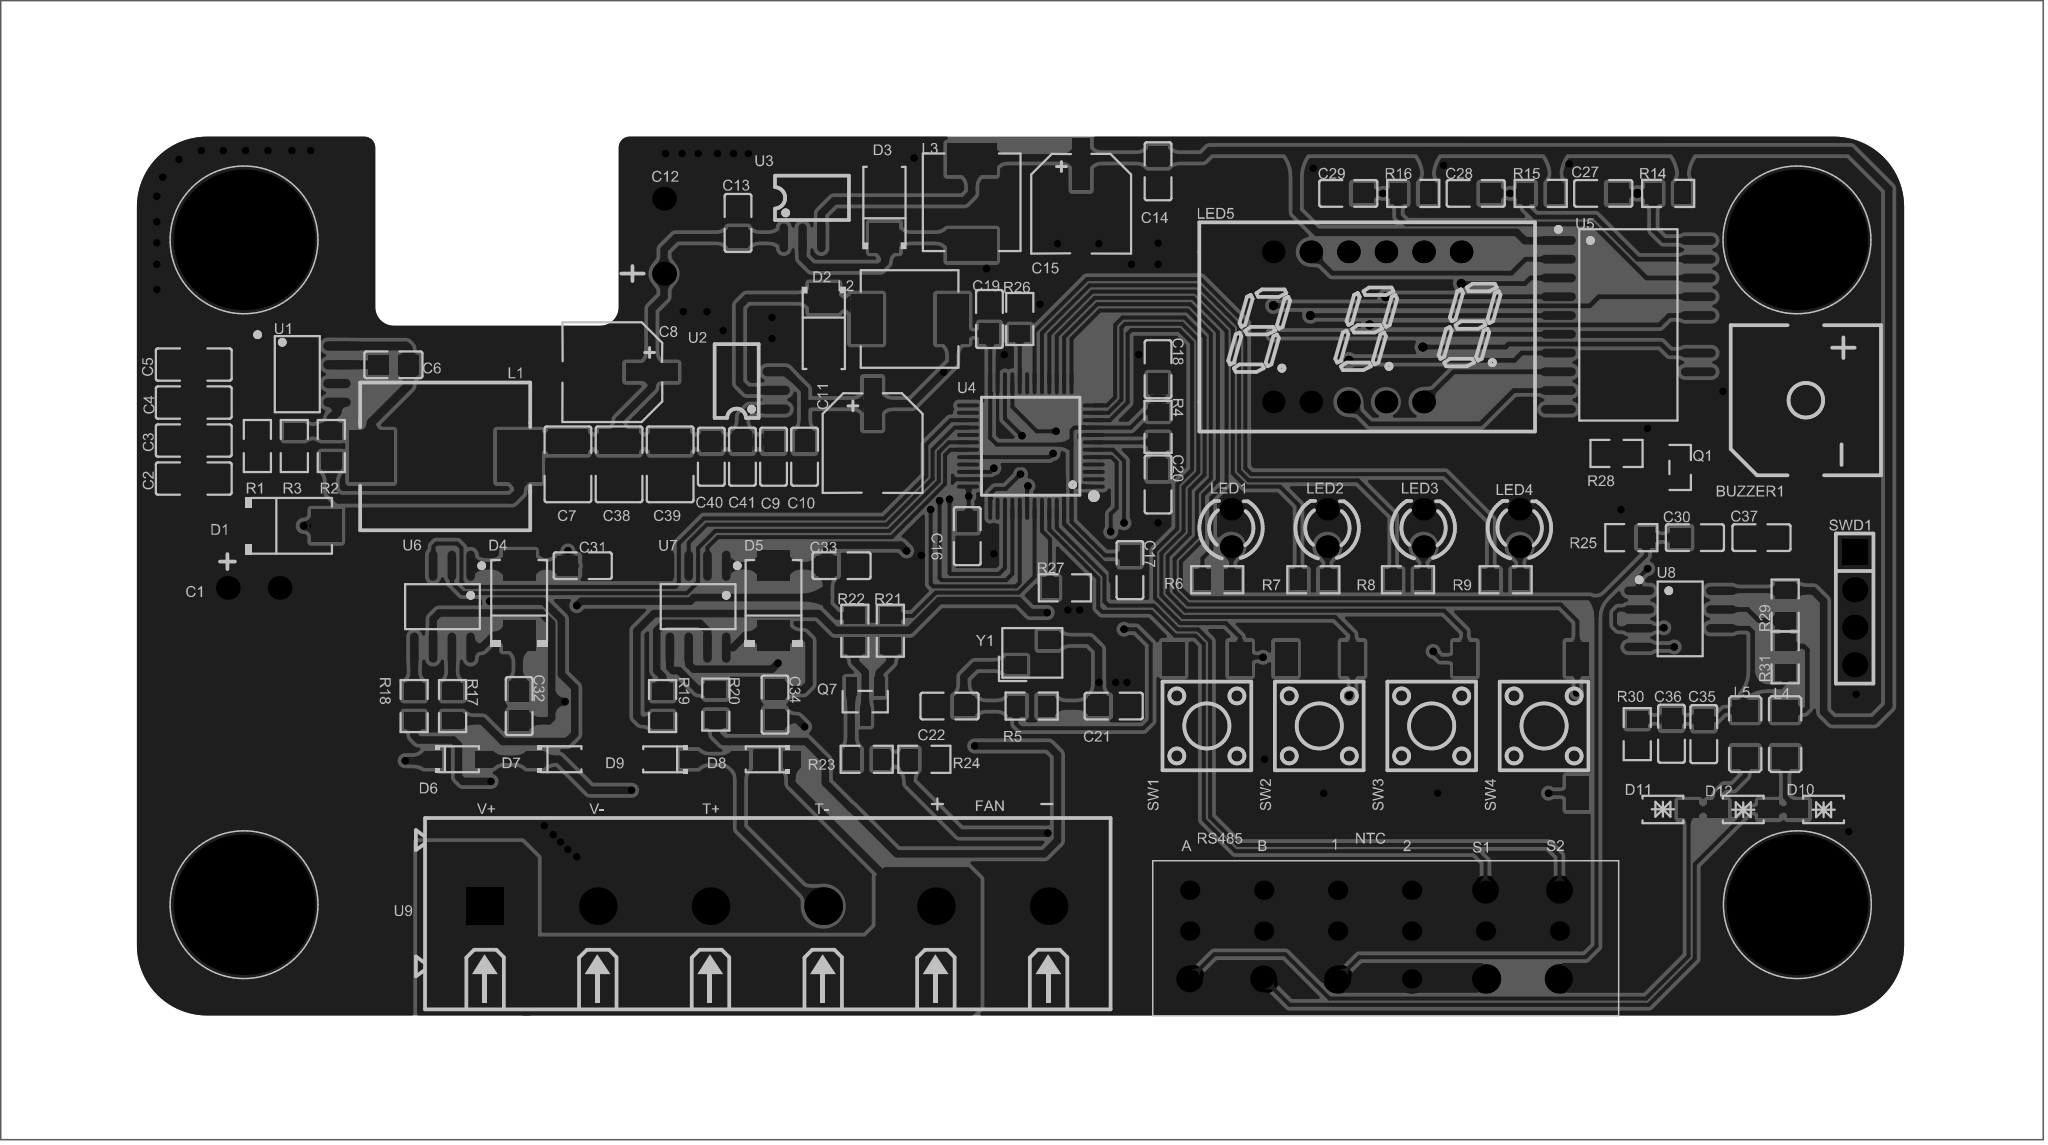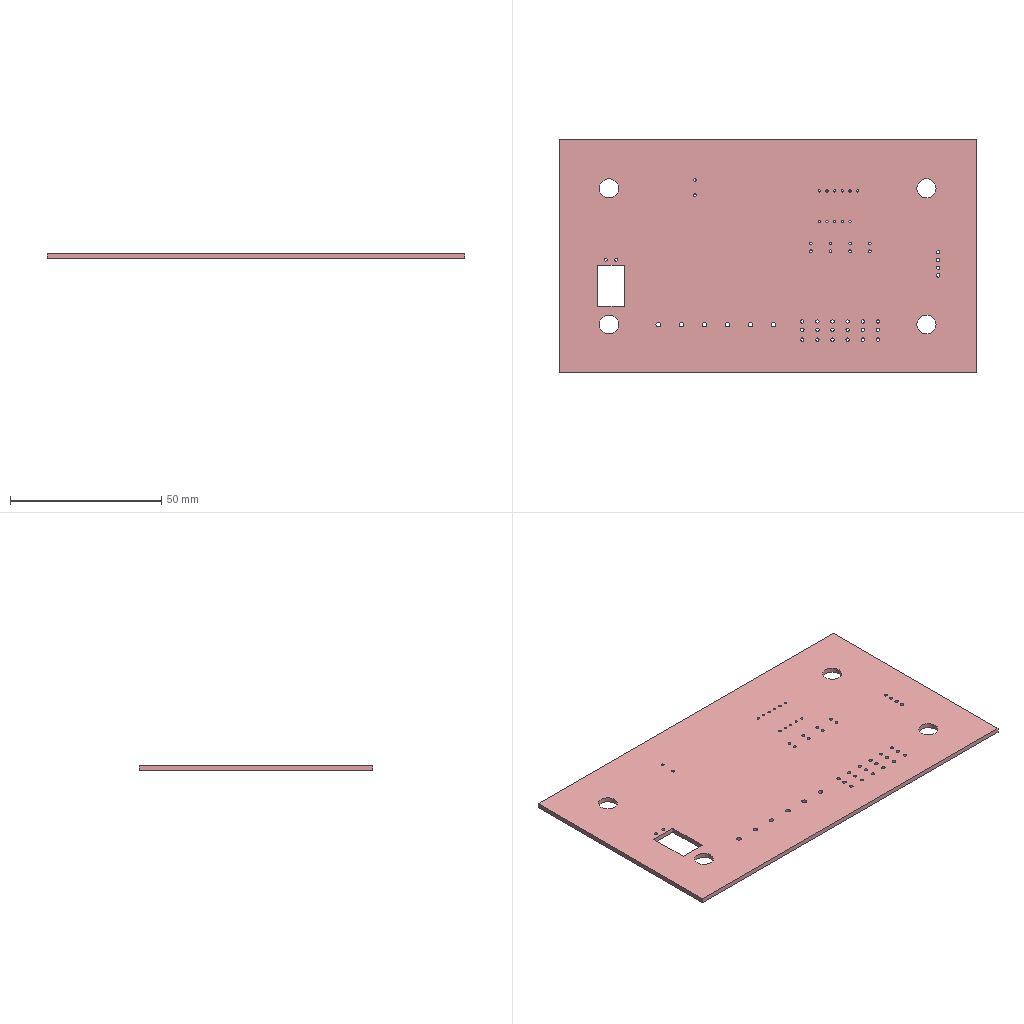Circuit board layout | Altium Designer | box 138.1 x 77.1 x 1.6 mm
Layer stack:
# Altium Designer layer stack of  (unit mm; dielectric type: 0 none, 1 core, 2 prepreg, 3 surface material)
index,name,kind,layer,copper_thickness_mm,dielectric_type,dielectric_thickness_mm,dielectric_material,dielectric_constant
0,Top Paste Mask Layer,other,,,,,,
1,Top Silkscreen Layer,other,,,,,,
2,Top Solder Mask Layer,dielectric,,,3,0.0102,,3.3
3,Top Layer,copper,Top Layer,0.0356,,,,
4,Dielectric1,dielectric,,,3,1.509,FR4,4.5
5,Bottom Layer,copper,Bottom Layer,0.0356,,,,
6,Bottom Solder Mask Layer,dielectric,,,3,0.0102,,3.3
7,Bottom Silkscreen Layer,other,,,,,,
8,Bottom Paste Mask Layer,other,,,,,,
# drill layer pairs: low layer,high layer
drill_pair,Top Layer,Bottom Layer
Part placement:
Designator,Comment,Layer,Footprint,Center-X(mm),Center-Y(mm),Rotation
BUZZER1,2.7kHz,TopLayer,BUZ-SMD_L9.6-W9.6-LS10.0-R,191.899,119.901,90
R30,47kΩ,TopLayer,R0805,180.5,97.3,90
C1,33uF,TopLayer,CAP-TH_BD8.0-P3.50-D1.0-FD,86.954,107.201,0
C2,2.2uF,TopLayer,C1206,82.9,114.6,0
C3,2.2uF,TopLayer,C1206,82.9,117.173,0
C4,100nF,TopLayer,C1206,82.9,119.743,0
C5,100nF,TopLayer,C1206,82.9,122.316,0
C6,100nF,TopLayer,C0805,96.399,122.301,0
C7,22uF,TopLayer,C1210,108.199,115.561,90
C8,100uF,TopLayer,CAP-SMD_BD6.3-L6.6-W6.6-LS7.3-FD_JVS25V100M6X4,111.2,121.801,180
C9,100nF,TopLayer,C0805,122.1,116.079,270
C10,100nF,TopLayer,C0805,124.201,116.079,90
C11,100uF,TopLayer,CAP-SMD_BD6.3-L6.6-W6.6-LS7.3-FD_JVS25V100M6X4,128.801,117,270
C13,100nF,TopLayer,C0805,119.7,131.9,90
C14,100nF,TopLayer,C0805,148.1,135.4,90
C15,100uF,TopLayer,CAP-SMD_BD6.3-L6.6-W6.6-LS7.3-FD_JVS25V100M6X4,142.9,133.2,270
C16,100nF,TopLayer,C0805,135.199,110.7,90
C17,100nF,TopLayer,C0805,146.2,108.4,90
C19,100nF,TopLayer,C0805,136.7,125.4,270
C20,100nF,TopLayer,C0805,148.1,114.2,90
C21,22pF,TopLayer,C0805,145.1,99.2,0
C22,22pF,TopLayer,C0805,134,99.2,180
C23,100nF,BottomLayer,C0805,159.101,100.498,270
C24,100nF,BottomLayer,C0805,164.12,100.498,270
C25,100nF,BottomLayer,C0805,169.136,100.498,270
C26,100nF,BottomLayer,C0805,174.155,100.498,270
C28,100pF,TopLayer,C0805,169.582,133.901,180
C29,100pF,TopLayer,C0805,160.962,133.901,0
C30,100nF,TopLayer,C0805,184.399,110.599,0
C31,10uF,TopLayer,C0805,109.2,108.699,180
C32,10uF,TopLayer,C0805,104.9,99.2,90
C33,10uF,TopLayer,C0805,126.7,108.699,180
C34,10uF,TopLayer,C0805,122.199,99.3,90
C35,100nF,TopLayer,C0805,185.001,97.3,90
C37,100nF,TopLayer,C0805,188.9,110.599,0
C27,100pF,TopLayer,C0805,178.2,133.901,180
D2,SS34,TopLayer,SMA_L4.3-W2.6-LS5.2-RD,125.499,124.612,270
D3,SS34,TopLayer,SMA_L4.3-W2.6-LS5.2-RD,129.601,133.1,90
D4,MUR160SB,TopLayer,SMB_L4.6-W3.6-LS5.3-RD,104.9,106.338,90
D5,MUR160SB,TopLayer,SMB_L4.6-W3.6-LS5.3-RD,122.1,106.338,90
D6,RB160M-90,TopLayer,SOD-123FL_L2.7-W1.8-LS3.7-RD,100.8,95.6,0
D7,RB160M-90,TopLayer,SOD-123FL_L2.7-W1.8-LS3.7-RD,107.734,95.6,0
D8,RB160M-90,TopLayer,SOD-123FL_L2.7-W1.8-LS3.7-RD,121.6,95.593,180
D9,RB160M-90,TopLayer,SOD-123FL_L2.7-W1.8-LS3.7-RD,114.666,95.593,180
D10,SMF36CA,TopLayer,SOD-123_L2.7-W1.8-LS3.7-BI,193.101,92.2,0
D11,SMF36CA,TopLayer,SOD-123_L2.7-W1.8-LS3.7-BI,182.235,92.2,180
D12,SMF36CA,TopLayer,SOD-123_L2.7-W1.8-LS3.7-BI,187.668,92.2,0
LED1,3mmFIR,TopLayer,LED-TH_BD3.0-P2.54-FD,153.05,111.254,90
LED2,3mmFIR,TopLayer,LED-TH_BD3.0-P2.54-FD,159.55,111.254,90
LED3,3mmFIR,TopLayer,LED-TH_BD3.0-P2.54-FD,166.05,111.254,90
LED4,3mmFIR,TopLayer,LED-TH_BD3.0-P2.54-FD,172.55,111.254,90
Q1,SS8050(RANGE:200-350),TopLayer,SOT-23-3_L2.9-W1.3-P1.90-LS2.4-BR,183.399,115.349,180
Q2,NCE0140K2-VB,BottomLayer,TO-252-3_L6.6-W6.1-P4.58-LS10.1-BR,144.901,97.701,90
Q7,SS8050(RANGE:200-350),TopLayer,SOT-23-3_L2.9-W1.3-P1.90-LS2.4-BR,128.3,99.501,90
R2,100kΩ,TopLayer,R0805,92.2,116.801,270
R3,24.9kΩ,TopLayer,R0805,89.7,116.801,90
R4,10K,TopLayer,R0805,148.1,118.1,90
R5,1MΩ,TopLayer,R0805,139.55,99.2,0
R6,100Ω,TopLayer,R0805,152.1,107.749,180
R7,100Ω,TopLayer,R0805,158.6,107.749,180
R8,100Ω,TopLayer,R0805,165,107.749,180
R9,100Ω,TopLayer,R0805,171.6,107.749,180
R10,4.7kΩ,BottomLayer,R0805,159.101,95.998,270
R11,4.7kΩ,BottomLayer,R0805,164.12,95.998,270
R12,4.7kΩ,BottomLayer,R0805,169.136,95.998,270
R13,4.7kΩ,BottomLayer,R0805,174.155,95.998,270
R14,10K,TopLayer,R0805,182.59,133.901,0
R15,10K,TopLayer,R0805,173.972,133.901,0
R16,10K,TopLayer,R0805,165.353,133.901,0
R17,10Ω,TopLayer,R0805,100.401,99.2,270
R18,10Ω,TopLayer,R0805,97.8,99.2,270
R19,10Ω,TopLayer,R0805,114.6,99.2,270
R20,10Ω,TopLayer,R0805,118.199,99.3,270
R21,1kΩ,TopLayer,R0805,130,104.3,270
R23,10Ω,TopLayer,R0805,128.399,95.595,0
R24,10K,TopLayer,R0805,132.3,95.595,0
R25,10K,TopLayer,R0805,180.1,110.599,180
R26,10K,TopLayer,R0805,138.75,125.4,90
R27,10K,TopLayer,R0805,141.799,107.201,0
R28,1kΩ,TopLayer,R0805,179.101,116.299,0
R29,47kΩ,TopLayer,R0805,190.5,106.001,90
SW1,1TS005F-2600-9000A2-CT,TopLayer,SW-SMD_4P-L6.0-W6.0-P4.50-LS9.0-2,151.4,97.853,90
SW2,1TS005F-2600-9000A2-CT,TopLayer,SW-SMD_4P-L6.0-W6.0-P4.50-LS9.0-2,159,97.853,90
SW3,1TS005F-2600-9000A2-CT,TopLayer,SW-SMD_4P-L6.0-W6.0-P4.50-LS9.0-2,166.6,97.853,90
SW4,1TS005F-2600-9000A2-CT,TopLayer,SW-SMD_4P-L6.0-W6.0-P4.50-LS9.0-2,174.201,97.853,90
SWD1,220S-1*4P H=8.5MM Ytype Gold-plated,TopLayer,DIP-1X4P2.54,195.199,105.801,270
C36,100nF,TopLayer,C0805,182.816,97.326,270
U1,LMR38020SDDAR,TopLayer,ESOP-8_L4.9-W3.9-P1.27-LS6.0-BL-EP-1,89.901,121.666,270
U2,XL1509-3.3E1,TopLayer,SOP-8_L4.9-W3.9-P1.27-LS6.0-BL,119.601,121.201,90
U3,XL1509-5.0E1,TopLayer,SOIC-8_L5.0-W4.0-P1.27-LS6.0-BL,124.699,133.599,0
U4,STM32F103C8T6,TopLayer,LQFP-48_L7.0-W7.0-P0.50-LS9.0-BL,139.499,116.799,90
U5,TM1620,TopLayer,SOIC-20_L13.0-W7.6-P1.27-LS10.3-BL,179.901,125.001,270
U6,IR2103STRPBF,TopLayer,SOIC-8_L4.9-W3.9-P1.27-LS6.0-BL,99.718,105.927,180
U7,IR2103STRPBF,TopLayer,SOIC-8_L4.9-W3.9-P1.27-LS6.0-BL,117,105.927,180
U8,MAX485ESA(UMW),TopLayer,SOP-8_L5.0-W4.0-P1.27-LS6.0-BL,183.399,105.1,270
C18,100nF,TopLayer,C0805,148.1,122,270
R22,4.7kΩ,TopLayer,R0805,127.599,104.3,90
U9,KF7620-7.62-6P,TopLayer,CONN-TH_6P-P7.62_KF7620-7.62-6P,121.651,85.654,0
L2,68uH,TopLayer,IND-SMD_L7.1-W6.6_H5.0,131.3,125.4,180
L3,68uH,TopLayer,IND-SMD_L7.1-W6.6_H5.0,135.499,133.3,270
LED5,SP420361N,TopLayer,LED-SEG-TH_SP420361N,162.24,124.864,270
R1,64.9kΩ,TopLayer,R0805,87.201,116.801,90
L4,22uH,TopLayer,L1206,190.5,97.3,270
L5,22uH,TopLayer,L1206,187.8,97.3,270
C12,470uF,TopLayer,CAP-TH_BD10.0-P5.00-D1.0-FD,114.699,131,0
Q3,HYG025N06LS1B,BottomLayer,TO-263-2_L10.2-W8.7-P5.08-LS15.1-BR,108.599,108.9,180
Q4,HYG025N06LS1B,BottomLayer,TO-263-2_L10.2-W8.7-P5.08-LS15.1-BR,108.599,96.599,180
Q5,HYG025N06LS1B,BottomLayer,TO-263-2_L10.2-W8.7-P5.08-LS15.1-BR,130.001,108.9,0
Q6,HYG025N06LS1B,BottomLayer,TO-263-2_L10.2-W8.7-P5.08-LS15.1-BR,130.001,96.599,0
C38,22uF,TopLayer,C1210,111.656,115.561,90
C39,22uF,TopLayer,C1210,115.113,115.561,90
C40,100nF,TopLayer,C0805,117.894,116.079,90
C41,1nF,TopLayer,C0805,120,116.079,90
R31,120Ω,TopLayer,R0805,190.5,102.5,90
L1,33uH,TopLayer,IND-SMD_L11.5-W10.0_FXL1040,99.9,116.101,0
D1,US2M-TP,TopLayer,SMB_L4.6-W3.6-LS5.3-RD,89.501,111.399,0
Y1,8MHz,TopLayer,CRYSTAL-SMD_4P-L3.2-W2.5-BL,139.601,102.8,0
Pad and via stacks:
# Altium Designer via and pad stacks of  (unit mm). Each distinct definition once, with the count of objects using it.
# via: kind,start_layer,end_layer,hole_mm,diameter_mm,mode(0 simple;1 top-mid-bottom;2 full stack),diameter_per_layer,count,example_net
# pad: kind,layer,hole_mm,hole_type(0 round;1 square;2 slot),plating,top_size,top_shape(1 round;2 rect;3 octagon;9 rounded rect),mid_size,bottom_size,mode,footprint,size_per_layer,count,example
pad,Top Layer,0,0,plated,2.499x1.801,2,2.499x1.801,2.499x1.801,0,BUZ-SMD_L9.6-W9.6-LS10.0-R,,2,BUZZER1.1
pad,Top Layer,0,0,plated,1.133x1.377,2,1.133x1.377,1.133x1.377,0,R0805,,54,R30.2
pad,Top Layer,0,0,plated,1.486x1.727,2,1.486x1.727,1.486x1.727,0,C1206,,8,C2.2
pad,Top Layer,0,0,plated,1.41x1.349,2,1.41x1.349,1.41x1.349,0,C0805,,50,C6.2
pad,Top Layer,0,0,plated,1.636x2.7,2,1.636x2.7,1.636x2.7,0,C1210,,6,C7.2
pad,Top Layer,0,0,plated,3.5x1.199,2,3.5x1.199,3.5x1.199,0,CAP-SMD_BD6.3-L6.6-W6.6-LS7.3-FD_JVS25V100M6X4,,6,C8.1
pad,Top Layer,0,0,plated,1.999x1.999,2,1.999x1.999,1.999x1.999,0,SMA_L4.3-W2.6-LS5.2-RD,,4,D2.2
pad,Top Layer,0,0,plated,2.047x2.192,2,2.047x2.192,2.047x2.192,0,SMB_L4.6-W3.6-LS5.3-RD,,6,D4.2
pad,Top Layer,0,0,plated,1.199x1.151,2,1.199x1.151,1.199x1.151,0,SOD-123FL_L2.7-W1.8-LS3.7-RD,,8,D6.2
pad,Top Layer,0,0,plated,1.399x1.199,2,1.399x1.199,1.399x1.199,0,SOD-123_L2.7-W1.8-LS3.7-BI,,6,D10.2
pad,Top Layer,0,0,plated,1.25x0.701,2,1.25x0.701,1.25x0.701,0,SOT-23-3_L2.9-W1.3-P1.90-LS2.4-BR,,6,Q1.1
pad,Top Layer,0,0,plated,2.301x1.501,2,2.301x1.501,2.301x1.501,0,SW-SMD_4P-L6.0-W6.0-P4.50-LS9.0-2,,16,SW1.1
pad,Top Layer,0,0,plated,0.6299x1.864,1,0.6299x1.864,0.6299x1.864,0,ESOP-8_L4.9-W3.9-P1.27-LS6.0-BL-EP-1,,8,U1.5
pad,Top Layer,0,0,plated,3.3x2.4,2,3.3x2.4,3.3x2.4,0,ESOP-8_L4.9-W3.9-P1.27-LS6.0-BL-EP-1,,1,U1.9
pad,Top Layer,0,0,plated,0.6299x1.864,1,0.6299x1.864,0.6299x1.864,0,SOP-8_L4.9-W3.9-P1.27-LS6.0-BL,,8,U2.1
pad,Top Layer,0,0,plated,0.569x1.951,1,0.569x1.951,0.569x1.951,0,SOIC-8_L5.0-W4.0-P1.27-LS6.0-BL,,8,U3.1
pad,Top Layer,0,0,plated,0.2692x1.501,1,0.2692x1.501,0.2692x1.501,0,LQFP-48_L7.0-W7.0-P0.50-LS9.0-BL,,24,U4.1
pad,Top Layer,0,0,plated,1.501x0.2692,1,1.501x0.2692,1.501x0.2692,0,LQFP-48_L7.0-W7.0-P0.50-LS9.0-BL,,24,U4.13
pad,Top Layer,0,0,plated,0.5944x2.36,1,0.5944x2.36,0.5944x2.36,0,SOIC-20_L13.0-W7.6-P1.27-LS10.3-BL,,20,U5.1
pad,Top Layer,0,0,plated,0.5867x2.045,1,0.5867x2.045,0.5867x2.045,0,SOIC-8_L4.9-W3.9-P1.27-LS6.0-BL,,16,U6.1
pad,Top Layer,0,0,plated,0.574x2.034,1,0.574x2.034,0.574x2.034,0,SOP-8_L5.0-W4.0-P1.27-LS6.0-BL,,8,U8.1
pad,Top Layer,0,0,plated,2.149x3.32,2,2.149x3.32,2.149x3.32,0,IND-SMD_L7.1-W6.6_H5.0,,4,L2.2
pad,Top Layer,0,0,plated,1.486x1.727,2,1.486x1.727,1.486x1.727,0,L1206,,4,L4.2
pad,Top Layer,0,0,plated,3x3.5,2,3x3.5,3x3.5,0,IND-SMD_L11.5-W10.0_FXL1040,,2,L1.1
pad,Top Layer,0,0,plated,1.399x1.199,2,1.399x1.199,1.399x1.199,0,CRYSTAL-SMD_4P-L3.2-W2.5-BL,,4,Y1.1
pad,Multi-Layer,1.001,0,plated,1.6x1.6,1,1.6x1.6,1.6x1.6,0,CAP-TH_BD8.0-P3.50-D1.0-FD,,2,C1.2
pad,Multi-Layer,0.9144,0,plated,1.524x1.524,1,1.524x1.524,1.524x1.524,0,LED-TH_BD3.0-P2.54-FD,,8,LED1.1
pad,Multi-Layer,1.1,0,plated,1.699x1.699,2,1.699x1.699,1.699x1.699,0,DIP-1X4P2.54,,1,SWD1.1
pad,Multi-Layer,1.1,0,plated,1.699x1.699,1,1.699x1.699,1.699x1.699,0,DIP-1X4P2.54,,3,SWD1.2
pad,Multi-Layer,1.501,0,plated,2.54x2.54,1,2.54x2.54,2.54x2.54,0,CONN-TH_6P-P7.62_KF7620-7.62-6P,,5,U9.6
pad,Multi-Layer,1.501,0,plated,2.54x2.54,2,2.54x2.54,2.54x2.54,0,CONN-TH_6P-P7.62_KF7620-7.62-6P,,1,U9.1
pad,Multi-Layer,1.143,0,plated,1.3x1.3,1,1.3x1.3,1.999x1.999,1,,,6,1
pad,Multi-Layer,1.1,0,plated,1.3x1.3,1,1.3x1.3,1.999x1.999,1,,,12,0
pad,Multi-Layer,0.762,0,plated,1.524x1.524,1,1.524x1.524,1.524x1.524,0,LED-SEG-TH_SP420361N,,11,LED5.1
pad,Multi-Layer,1.001,0,plated,1.6x1.6,1,1.6x1.6,1.6x1.6,0,CAP-TH_BD10.0-P5.00-D1.0-FD,,2,C12.1
pad,Multi-Layer,6.35,0,plated,9.5x9.5,1,9.5x9.5,9.5x9.5,0,,,4,1
pad,Bottom Layer,0,0,plated,1.41x1.349,2,1.41x1.349,1.41x1.349,0,C0805,,8,C23.2
pad,Bottom Layer,0,0,plated,6.5x6,2,6.5x6,6.5x6,0,TO-252-3_L6.6-W6.1-P4.58-LS10.1-BR,,1,Q2.3
pad,Bottom Layer,0,0,plated,3x1.6,2,3x1.6,3x1.6,0,TO-252-3_L6.6-W6.1-P4.58-LS10.1-BR,,2,Q2.1
pad,Bottom Layer,0,0,plated,1.133x1.377,2,1.133x1.377,1.133x1.377,0,R0805,,8,R10.2
pad,Bottom Layer,0,0,plated,8.839x11.001,2,8.839x11.001,8.839x11.001,0,TO-263-2_L10.2-W8.7-P5.08-LS15.1-BR,,4,Q3.4
pad,Bottom Layer,0,0,plated,3.81x1.999,2,3.81x1.999,3.81x1.999,0,TO-263-2_L10.2-W8.7-P5.08-LS15.1-BR,,8,Q3.3
via,Top Layer,Bottom Layer,0.3048,0.6096,0,,9,B
via,Top Layer,Bottom Layer,0.2997,0.5004,0,,157,CLK
Copper pours:
name,layer,net,type(0 solid;1 hatched;2 none)
Top Layer-VCC,Top Layer,VCC,0
Top Layer-GND,Top Layer,GND,0
Top Layer-VCC 1,Top Layer,VCC,0
Bottom Layer-VCC,Bottom Layer,VCC,0
Bottom Layer-T+,Bottom Layer,T+,0
Bottom Layer-T-,Bottom Layer,T-,0
Bottom Layer-GND,Bottom Layer,GND,0
Design rules, without the lines most boards share:
# Altium Designer design rules of  (exported by Altium Designer, unit mm)
# columns: name | kind | enabled | priority | scope1 | scope2 | descriptor | typed fields (field=value)
HoleToHoleClearance | 52 | enabled | 1 | All | All | Hole To Hole Clearance (Gap=10mil) (All),(All) | gap=0.254
copperThickness1oz | 0 | enabled | 2 | All | All | Clearance Constraint (Gap=7mil) (All),(All) | gap=0.1778
copperThickness2oz | 0 | enabled | 1 | All | All | Clearance Constraint (Gap=7mil) (All),(All) | gap=0.1778
copperThickness2oz_1 | 63 | enabled | 1 | All | All | Board Clearance Constraint (Gap=0mil) (All) |
Plane_innerPlane | 0 | enabled | 3 | All | All | Clearance Constraint (Gap=7mil) (All),(All) | gap=0.1778
Plane_innerPlane_1 | 63 | enabled | 3 | All | All | Board Clearance Constraint (Gap=0mil) (All) |
Copper_copperRegion | 0 | enabled | 5 | All | All | Clearance Constraint (Gap=7mil) (All),(All) | gap=0.1778
Copper_copperRegion_1 | 63 | enabled | 5 | All | All | Board Clearance Constraint (Gap=0mil) (All) |
otherClearance | 0 | enabled | 4 | All | All | Clearance Constraint (Gap=7mil) (All),(All) | gap=0.1778
otherClearance_1 | 63 | enabled | 4 | All | All | Board Clearance Constraint (Gap=0mil) (All) |
copperThickness1oz_2 | 2 | enabled | 1 | All | All | Width Constraint (Min=5mil) (Max=120mil) (Preferred=10mil) (All) |
copperThickness2oz_2 | 2 | enabled | 2 | All | All | Width Constraint (Min=8mil) (Max=100mil) (Preferred=10mil) (All) |
viaSize | 11 | enabled | 1 | All | All | Routing Via (MinHoleWidth=11.811mil) (MaxHoleWidth=248.031mil) (PreferredHoleWidth=11.811mil) (MinWidth=11.811mil) (MaxWidth=248.031mil) (PreferedWidth=11.811mil) (All) | via_min_hole=0.3 via_max_hole=6.3 via_preferred_diameter=0.3 via_preferred_hole=0.3
copperRegion | 20 | enabled | 1 | All | All | Polygon Connect Rule(Direct Connect )(Conductor Width=10mil) (Relief Angle=90 Angle) (Entries=4) (Air Gap Width=10mil) (All),(All) | connect_style(0=relief,1=direct,2=none)=1 relief_conductor_width=0.254 relief_entries=4